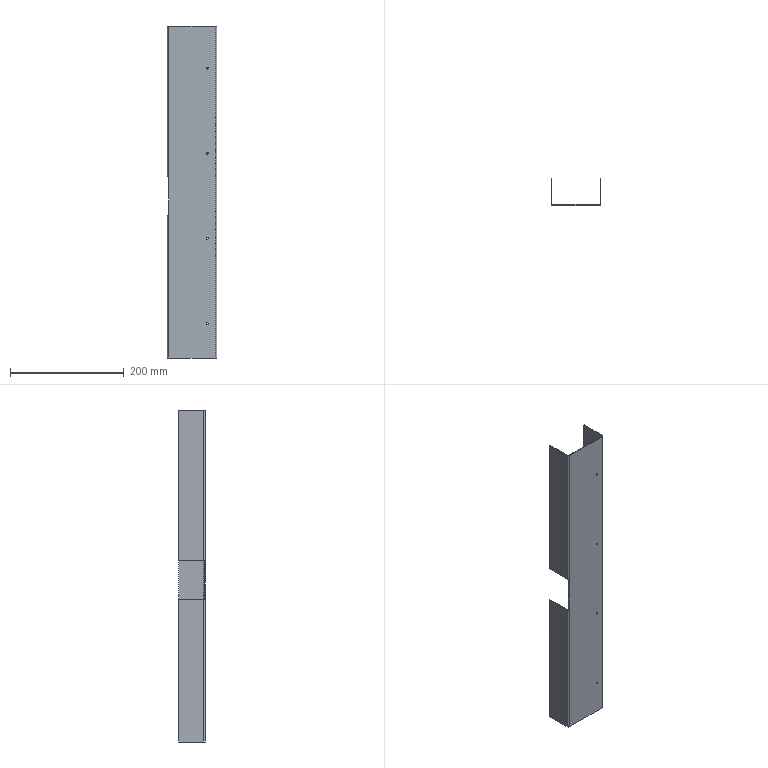Part | SolidWorks | features ICE 2, Cut 1, FlatPattern 1, SMBaseFlange 1, SheetMetal 1 | 1 solid | 38 faces | box 88 x 47.5 x 585 mm | volume 151349 mm3 | plane 24 | cylinder 14 | commonest cylinder face diameters 3 x11 6 x3
STEP:
#1=CARTESIAN_POINT('',(57.727,5.741,59.2));
#2=VERTEX_POINT('',#1);
#3=CARTESIAN_POINT('',(57.727,5.741,62.2));
#4=VERTEX_POINT('',#3);
#5=CARTESIAN_POINT('',(57.727,5.741,60.7));
#6=DIRECTION('',(0.,1.,0.));
#7=DIRECTION('',(0.,0.,1.));
#8=AXIS2_PLACEMENT_3D('',#5,#6,#7);
#9=CIRCLE('',#8,1.5);
#10=EDGE_CURVE('',#2,#4,#9,.T.);
#11=ORIENTED_EDGE('',*,*,#10,.T.);
#12=CARTESIAN_POINT('',(57.727,4.241,62.2));
#13=VERTEX_POINT('',#12);
#14=CARTESIAN_POINT('',(57.727,14.241,62.2));
#15=DIRECTION('',(0.,-1.,0.));
#16=VECTOR('',#15,1000.);
#17=LINE('',#14,#16);
#18=EDGE_CURVE('',#4,#13,#17,.T.);
#19=ORIENTED_EDGE('',*,*,#18,.T.);
#20=CARTESIAN_POINT('',(57.727,4.241,59.2));
#21=VERTEX_POINT('',#20);
#22=CARTESIAN_POINT('',(57.727,4.241,60.7));
#23=DIRECTION('',(0.,-1.,0.));
#24=DIRECTION('',(0.,0.,-1.));
#25=AXIS2_PLACEMENT_3D('',#22,#23,#24);
#26=CIRCLE('',#25,1.5);
#27=EDGE_CURVE('',#13,#21,#26,.T.);
#28=ORIENTED_EDGE('',*,*,#27,.T.);
#29=CARTESIAN_POINT('',(57.727,14.241,59.2));
#30=DIRECTION('',(0.,-1.,0.));
#31=VECTOR('',#30,1000.);
#32=LINE('',#29,#31);
#33=EDGE_CURVE('',#2,#21,#32,.T.);
#34=ORIENTED_EDGE('',*,*,#33,.F.);
#35=EDGE_LOOP('',(#11,#19,#28,#34));
#36=FACE_OUTER_BOUND('',#35,.T.);
#37=CARTESIAN_POINT('',(57.727,14.241,60.7));
#38=DIRECTION('',(0.,-1.,0.));
#39=DIRECTION('',(0.,0.,-1.));
#40=AXIS2_PLACEMENT_3D('',#37,#38,#39);
#41=CYLINDRICAL_SURFACE('',#40,1.5);
#42=ADVANCED_FACE('',(#36),#41,.F.);
#43=CARTESIAN_POINT('',(57.727,5.741,209.2));
#44=VERTEX_POINT('',#43);
#45=CARTESIAN_POINT('',(57.727,5.741,212.2));
#46=VERTEX_POINT('',#45);
#47=CARTESIAN_POINT('',(57.727,5.741,210.7));
#48=DIRECTION('',(0.,1.,0.));
#49=DIRECTION('',(0.,0.,1.));
#50=AXIS2_PLACEMENT_3D('',#47,#48,#49);
#51=CIRCLE('',#50,1.5);
#52=EDGE_CURVE('',#44,#46,#51,.T.);
#53=ORIENTED_EDGE('',*,*,#52,.T.);
#54=CARTESIAN_POINT('',(57.727,4.241,212.2));
#55=VERTEX_POINT('',#54);
#56=CARTESIAN_POINT('',(57.727,14.241,212.2));
#57=DIRECTION('',(0.,-1.,0.));
#58=VECTOR('',#57,1000.);
#59=LINE('',#56,#58);
#60=EDGE_CURVE('',#46,#55,#59,.T.);
#61=ORIENTED_EDGE('',*,*,#60,.T.);
#62=CARTESIAN_POINT('',(57.727,4.241,209.2));
#63=VERTEX_POINT('',#62);
#64=CARTESIAN_POINT('',(57.727,4.241,210.7));
#65=DIRECTION('',(0.,-1.,0.));
#66=DIRECTION('',(0.,0.,-1.));
#67=AXIS2_PLACEMENT_3D('',#64,#65,#66);
#68=CIRCLE('',#67,1.5);
#69=EDGE_CURVE('',#55,#63,#68,.T.);
#70=ORIENTED_EDGE('',*,*,#69,.T.);
#71=CARTESIAN_POINT('',(57.727,14.241,209.2));
#72=DIRECTION('',(0.,-1.,0.));
#73=VECTOR('',#72,1000.);
#74=LINE('',#71,#73);
#75=EDGE_CURVE('',#44,#63,#74,.T.);
#76=ORIENTED_EDGE('',*,*,#75,.F.);
#77=EDGE_LOOP('',(#53,#61,#70,#76));
#78=FACE_OUTER_BOUND('',#77,.T.);
#79=CARTESIAN_POINT('',(57.727,14.241,210.7));
#80=DIRECTION('',(0.,-1.,0.));
#81=DIRECTION('',(0.,0.,-1.));
#82=AXIS2_PLACEMENT_3D('',#79,#80,#81);
#83=CYLINDRICAL_SURFACE('',#82,1.5);
#84=ADVANCED_FACE('',(#78),#83,.F.);
#85=CARTESIAN_POINT('',(57.727,5.741,359.2));
#86=VERTEX_POINT('',#85);
#87=CARTESIAN_POINT('',(57.727,5.741,362.2));
#88=VERTEX_POINT('',#87);
#89=CARTESIAN_POINT('',(57.727,5.741,360.7));
#90=DIRECTION('',(0.,1.,0.));
#91=DIRECTION('',(0.,0.,1.));
#92=AXIS2_PLACEMENT_3D('',#89,#90,#91);
#93=CIRCLE('',#92,1.5);
#94=EDGE_CURVE('',#86,#88,#93,.T.);
#95=ORIENTED_EDGE('',*,*,#94,.T.);
#96=CARTESIAN_POINT('',(57.727,4.241,362.2));
#97=VERTEX_POINT('',#96);
#98=CARTESIAN_POINT('',(57.727,14.241,362.2));
#99=DIRECTION('',(0.,-1.,0.));
#100=VECTOR('',#99,1000.);
#101=LINE('',#98,#100);
#102=EDGE_CURVE('',#88,#97,#101,.T.);
#103=ORIENTED_EDGE('',*,*,#102,.T.);
#104=CARTESIAN_POINT('',(57.727,4.241,359.2));
#105=VERTEX_POINT('',#104);
#106=CARTESIAN_POINT('',(57.727,4.241,360.7));
#107=DIRECTION('',(0.,-1.,0.));
#108=DIRECTION('',(0.,0.,-1.));
#109=AXIS2_PLACEMENT_3D('',#106,#107,#108);
#110=CIRCLE('',#109,1.5);
#111=EDGE_CURVE('',#97,#105,#110,.T.);
#112=ORIENTED_EDGE('',*,*,#111,.T.);
#113=CARTESIAN_POINT('',(57.727,14.241,359.2));
#114=DIRECTION('',(0.,-1.,0.));
#115=VECTOR('',#114,1000.);
#116=LINE('',#113,#115);
#117=EDGE_CURVE('',#86,#105,#116,.T.);
#118=ORIENTED_EDGE('',*,*,#117,.F.);
#119=EDGE_LOOP('',(#95,#103,#112,#118));
#120=FACE_OUTER_BOUND('',#119,.T.);
#121=CARTESIAN_POINT('',(57.727,14.241,360.7));
#122=DIRECTION('',(0.,-1.,0.));
#123=DIRECTION('',(0.,0.,-1.));
#124=AXIS2_PLACEMENT_3D('',#121,#122,#123);
#125=CYLINDRICAL_SURFACE('',#124,1.5);
#126=ADVANCED_FACE('',(#120),#125,.F.);
#127=CARTESIAN_POINT('',(57.727,5.741,509.2));
#128=VERTEX_POINT('',#127);
#129=CARTESIAN_POINT('',(57.727,5.741,512.2));
#130=VERTEX_POINT('',#129);
#131=CARTESIAN_POINT('',(57.727,5.741,510.7));
#132=DIRECTION('',(0.,1.,0.));
#133=DIRECTION('',(0.,0.,1.));
#134=AXIS2_PLACEMENT_3D('',#131,#132,#133);
#135=CIRCLE('',#134,1.5);
#136=EDGE_CURVE('',#128,#130,#135,.T.);
#137=ORIENTED_EDGE('',*,*,#136,.T.);
#138=CARTESIAN_POINT('',(57.727,4.241,512.2));
#139=VERTEX_POINT('',#138);
#140=CARTESIAN_POINT('',(57.727,14.241,512.2));
#141=DIRECTION('',(0.,-1.,0.));
#142=VECTOR('',#141,1000.);
#143=LINE('',#140,#142);
#144=EDGE_CURVE('',#130,#139,#143,.T.);
#145=ORIENTED_EDGE('',*,*,#144,.T.);
#146=CARTESIAN_POINT('',(57.727,4.241,509.2));
#147=VERTEX_POINT('',#146);
#148=CARTESIAN_POINT('',(57.727,4.241,510.7));
#149=DIRECTION('',(0.,-1.,0.));
#150=DIRECTION('',(0.,0.,-1.));
#151=AXIS2_PLACEMENT_3D('',#148,#149,#150);
#152=CIRCLE('',#151,1.5);
#153=EDGE_CURVE('',#139,#147,#152,.T.);
#154=ORIENTED_EDGE('',*,*,#153,.T.);
#155=CARTESIAN_POINT('',(57.727,14.241,509.2));
#156=DIRECTION('',(0.,-1.,0.));
#157=VECTOR('',#156,1000.);
#158=LINE('',#155,#157);
#159=EDGE_CURVE('',#128,#147,#158,.T.);
#160=ORIENTED_EDGE('',*,*,#159,.F.);
#161=EDGE_LOOP('',(#137,#145,#154,#160));
#162=FACE_OUTER_BOUND('',#161,.T.);
#163=CARTESIAN_POINT('',(57.727,14.241,510.7));
#164=DIRECTION('',(0.,-1.,0.));
#165=DIRECTION('',(0.,0.,-1.));
#166=AXIS2_PLACEMENT_3D('',#163,#164,#165);
#167=CYLINDRICAL_SURFACE('',#166,1.5);
#168=ADVANCED_FACE('',(#162),#167,.F.);
#169=CARTESIAN_POINT('',(-13.373,7.241,319.25));
#170=VERTEX_POINT('',#169);
#171=CARTESIAN_POINT('',(-10.373,4.241,319.25));
#172=VERTEX_POINT('',#171);
#173=CARTESIAN_POINT('',(-10.373,7.241,319.25));
#174=DIRECTION('',(0.,0.,1.));
#175=DIRECTION('',(1.,0.,0.));
#176=AXIS2_PLACEMENT_3D('',#173,#174,#175);
#177=CIRCLE('',#176,3.);
#178=EDGE_CURVE('',#170,#172,#177,.T.);
#179=ORIENTED_EDGE('',*,*,#178,.T.);
#180=CARTESIAN_POINT('',(-10.373,4.241,585.));
#181=VERTEX_POINT('',#180);
#182=CARTESIAN_POINT('',(-10.373,4.241,585.));
#183=DIRECTION('',(0.,0.,-1.));
#184=VECTOR('',#183,1000.);
#185=LINE('',#182,#184);
#186=EDGE_CURVE('',#181,#172,#185,.T.);
#187=ORIENTED_EDGE('',*,*,#186,.F.);
#188=CARTESIAN_POINT('',(-13.373,7.241,585.));
#189=VERTEX_POINT('',#188);
#190=CARTESIAN_POINT('',(-10.373,7.241,585.));
#191=DIRECTION('',(0.,0.,1.));
#192=DIRECTION('',(1.,0.,0.));
#193=AXIS2_PLACEMENT_3D('',#190,#191,#192);
#194=CIRCLE('',#193,3.);
#195=EDGE_CURVE('',#189,#181,#194,.T.);
#196=ORIENTED_EDGE('',*,*,#195,.F.);
#197=CARTESIAN_POINT('',(-13.373,7.241,585.));
#198=DIRECTION('',(0.,0.,-1.));
#199=VECTOR('',#198,1000.);
#200=LINE('',#197,#199);
#201=EDGE_CURVE('',#189,#170,#200,.T.);
#202=ORIENTED_EDGE('',*,*,#201,.T.);
#203=EDGE_LOOP('',(#179,#187,#196,#202));
#204=FACE_OUTER_BOUND('',#203,.T.);
#205=CARTESIAN_POINT('',(-10.373,7.241,585.));
#206=DIRECTION('',(0.,0.,-1.));
#207=DIRECTION('',(-1.,0.,0.));
#208=AXIS2_PLACEMENT_3D('',#205,#206,#207);
#209=CYLINDRICAL_SURFACE('',#208,3.);
#210=ADVANCED_FACE('',(#204),#209,.T.);
#211=CARTESIAN_POINT('',(-10.373,5.741,251.75));
#212=VERTEX_POINT('',#211);
#213=CARTESIAN_POINT('',(-11.873,7.241,251.75));
#214=VERTEX_POINT('',#213);
#215=CARTESIAN_POINT('',(-10.373,7.241,251.75));
#216=DIRECTION('',(0.,0.,-1.));
#217=DIRECTION('',(-1.,0.,0.));
#218=AXIS2_PLACEMENT_3D('',#215,#216,#217);
#219=CIRCLE('',#218,1.5);
#220=EDGE_CURVE('',#212,#214,#219,.T.);
#221=ORIENTED_EDGE('',*,*,#220,.F.);
#222=CARTESIAN_POINT('',(-10.373,5.741,0.));
#223=VERTEX_POINT('',#222);
#224=CARTESIAN_POINT('',(-10.373,5.741,585.));
#225=DIRECTION('',(0.,0.,-1.));
#226=VECTOR('',#225,1000.);
#227=LINE('',#224,#226);
#228=EDGE_CURVE('',#212,#223,#227,.T.);
#229=ORIENTED_EDGE('',*,*,#228,.T.);
#230=CARTESIAN_POINT('',(-11.873,7.241,0.));
#231=VERTEX_POINT('',#230);
#232=CARTESIAN_POINT('',(-10.373,7.241,0.));
#233=DIRECTION('',(0.,0.,1.));
#234=DIRECTION('',(-1.,0.,0.));
#235=AXIS2_PLACEMENT_3D('',#232,#233,#234);
#236=CIRCLE('',#235,1.5);
#237=EDGE_CURVE('',#231,#223,#236,.T.);
#238=ORIENTED_EDGE('',*,*,#237,.F.);
#239=CARTESIAN_POINT('',(-11.873,7.241,585.));
#240=DIRECTION('',(0.,0.,-1.));
#241=VECTOR('',#240,1000.);
#242=LINE('',#239,#241);
#243=EDGE_CURVE('',#214,#231,#242,.T.);
#244=ORIENTED_EDGE('',*,*,#243,.F.);
#245=EDGE_LOOP('',(#221,#229,#238,#244));
#246=FACE_OUTER_BOUND('',#245,.T.);
#247=CARTESIAN_POINT('',(-10.373,7.241,585.));
#248=DIRECTION('',(0.,0.,-1.));
#249=DIRECTION('',(-1.,0.,0.));
#250=AXIS2_PLACEMENT_3D('',#247,#248,#249);
#251=CYLINDRICAL_SURFACE('',#250,1.5);
#252=ADVANCED_FACE('',(#246),#251,.F.);
#253=CARTESIAN_POINT('',(-11.873,51.741,251.75));
#254=VERTEX_POINT('',#253);
#255=CARTESIAN_POINT('',(-11.873,51.741,251.75));
#256=DIRECTION('',(0.,1.,0.));
#257=VECTOR('',#256,1000.);
#258=LINE('',#255,#257);
#259=EDGE_CURVE('',#214,#254,#258,.T.);
#260=ORIENTED_EDGE('',*,*,#259,.F.);
#261=ORIENTED_EDGE('',*,*,#243,.T.);
#262=CARTESIAN_POINT('',(-11.873,51.741,0.));
#263=VERTEX_POINT('',#262);
#264=CARTESIAN_POINT('',(-11.873,51.741,0.));
#265=DIRECTION('',(0.,-1.,0.));
#266=VECTOR('',#265,1000.);
#267=LINE('',#264,#266);
#268=EDGE_CURVE('',#263,#231,#267,.T.);
#269=ORIENTED_EDGE('',*,*,#268,.F.);
#270=CARTESIAN_POINT('',(-11.873,51.741,585.));
#271=DIRECTION('',(0.,0.,-1.));
#272=VECTOR('',#271,1000.);
#273=LINE('',#270,#272);
#274=EDGE_CURVE('',#254,#263,#273,.T.);
#275=ORIENTED_EDGE('',*,*,#274,.F.);
#276=EDGE_LOOP('',(#260,#261,#269,#275));
#277=FACE_OUTER_BOUND('',#276,.T.);
#278=CARTESIAN_POINT('',(-11.873,51.741,585.));
#279=DIRECTION('',(1.,0.,0.));
#280=DIRECTION('',(0.,1.,0.));
#281=AXIS2_PLACEMENT_3D('',#278,#279,#280);
#282=PLANE('',#281);
#283=ADVANCED_FACE('',(#277),#282,.T.);
#284=CARTESIAN_POINT('',(-13.373,51.741,251.75));
#285=VERTEX_POINT('',#284);
#286=CARTESIAN_POINT('',(-110.672,51.741,251.75));
#287=DIRECTION('',(-1.,0.,0.));
#288=VECTOR('',#287,1000.);
#289=LINE('',#286,#288);
#290=EDGE_CURVE('',#254,#285,#289,.T.);
#291=ORIENTED_EDGE('',*,*,#290,.F.);
#292=ORIENTED_EDGE('',*,*,#274,.T.);
#293=CARTESIAN_POINT('',(-13.373,51.741,0.));
#294=VERTEX_POINT('',#293);
#295=CARTESIAN_POINT('',(-13.373,51.741,0.));
#296=DIRECTION('',(1.,0.,0.));
#297=VECTOR('',#296,1000.);
#298=LINE('',#295,#297);
#299=EDGE_CURVE('',#294,#263,#298,.T.);
#300=ORIENTED_EDGE('',*,*,#299,.F.);
#301=CARTESIAN_POINT('',(-13.373,51.741,585.));
#302=DIRECTION('',(0.,0.,-1.));
#303=VECTOR('',#302,1000.);
#304=LINE('',#301,#303);
#305=EDGE_CURVE('',#285,#294,#304,.T.);
#306=ORIENTED_EDGE('',*,*,#305,.F.);
#307=EDGE_LOOP('',(#291,#292,#300,#306));
#308=FACE_OUTER_BOUND('',#307,.T.);
#309=CARTESIAN_POINT('',(-13.373,51.741,585.));
#310=DIRECTION('',(0.,1.,0.));
#311=DIRECTION('',(0.,0.,1.));
#312=AXIS2_PLACEMENT_3D('',#309,#310,#311);
#313=PLANE('',#312);
#314=ADVANCED_FACE('',(#308),#313,.T.);
#315=CARTESIAN_POINT('',(-13.373,7.241,251.75));
#316=VERTEX_POINT('',#315);
#317=CARTESIAN_POINT('',(-13.373,7.241,0.));
#318=VERTEX_POINT('',#317);
#319=CARTESIAN_POINT('',(-13.373,7.241,585.));
#320=DIRECTION('',(0.,0.,-1.));
#321=VECTOR('',#320,1000.);
#322=LINE('',#319,#321);
#323=EDGE_CURVE('',#316,#318,#322,.T.);
#324=ORIENTED_EDGE('',*,*,#323,.F.);
#325=CARTESIAN_POINT('',(-13.373,51.741,251.75));
#326=DIRECTION('',(0.,1.,0.));
#327=VECTOR('',#326,1000.);
#328=LINE('',#325,#327);
#329=EDGE_CURVE('',#316,#285,#328,.T.);
#330=ORIENTED_EDGE('',*,*,#329,.T.);
#331=ORIENTED_EDGE('',*,*,#305,.T.);
#332=CARTESIAN_POINT('',(-13.373,51.741,0.));
#333=DIRECTION('',(0.,-1.,0.));
#334=VECTOR('',#333,1000.);
#335=LINE('',#332,#334);
#336=EDGE_CURVE('',#294,#318,#335,.T.);
#337=ORIENTED_EDGE('',*,*,#336,.T.);
#338=EDGE_LOOP('',(#324,#330,#331,#337));
#339=FACE_OUTER_BOUND('',#338,.T.);
#340=CARTESIAN_POINT('',(-13.373,51.741,585.));
#341=DIRECTION('',(1.,0.,0.));
#342=DIRECTION('',(0.,1.,0.));
#343=AXIS2_PLACEMENT_3D('',#340,#341,#342);
#344=PLANE('',#343);
#345=ADVANCED_FACE('',(#339),#344,.F.);
#346=CARTESIAN_POINT('',(-10.373,5.741,585.));
#347=VERTEX_POINT('',#346);
#348=CARTESIAN_POINT('',(-10.373,5.741,585.));
#349=DIRECTION('',(0.,-1.,0.));
#350=VECTOR('',#349,1000.);
#351=LINE('',#348,#350);
#352=EDGE_CURVE('',#347,#181,#351,.T.);
#353=ORIENTED_EDGE('',*,*,#352,.F.);
#354=CARTESIAN_POINT('',(-11.873,7.241,585.));
#355=VERTEX_POINT('',#354);
#356=CARTESIAN_POINT('',(-10.373,7.241,585.));
#357=DIRECTION('',(0.,0.,1.));
#358=DIRECTION('',(-1.,0.,0.));
#359=AXIS2_PLACEMENT_3D('',#356,#357,#358);
#360=CIRCLE('',#359,1.5);
#361=EDGE_CURVE('',#355,#347,#360,.T.);
#362=ORIENTED_EDGE('',*,*,#361,.F.);
#363=CARTESIAN_POINT('',(-13.373,7.241,585.));
#364=DIRECTION('',(1.,0.,0.));
#365=VECTOR('',#364,1000.);
#366=LINE('',#363,#365);
#367=EDGE_CURVE('',#189,#355,#366,.T.);
#368=ORIENTED_EDGE('',*,*,#367,.F.);
#369=ORIENTED_EDGE('',*,*,#195,.T.);
#370=EDGE_LOOP('',(#353,#362,#368,#369));
#371=FACE_OUTER_BOUND('',#370,.T.);
#372=CARTESIAN_POINT('',(-10.373,5.741,585.));
#373=DIRECTION('',(0.,0.,1.));
#374=DIRECTION('',(1.,0.,0.));
#375=AXIS2_PLACEMENT_3D('',#372,#373,#374);
#376=PLANE('',#375);
#377=ADVANCED_FACE('',(#371),#376,.T.);
#378=CARTESIAN_POINT('',(71.627,5.741,585.));
#379=VERTEX_POINT('',#378);
#380=CARTESIAN_POINT('',(-11.873,5.741,585.));
#381=DIRECTION('',(1.,0.,0.));
#382=VECTOR('',#381,1000.);
#383=LINE('',#380,#382);
#384=EDGE_CURVE('',#347,#379,#383,.T.);
#385=ORIENTED_EDGE('',*,*,#384,.F.);
#386=ORIENTED_EDGE('',*,*,#352,.T.);
#387=CARTESIAN_POINT('',(71.627,4.241,585.));
#388=VERTEX_POINT('',#387);
#389=CARTESIAN_POINT('',(-11.873,4.241,585.));
#390=DIRECTION('',(1.,0.,0.));
#391=VECTOR('',#390,1000.);
#392=LINE('',#389,#391);
#393=EDGE_CURVE('',#181,#388,#392,.T.);
#394=ORIENTED_EDGE('',*,*,#393,.T.);
#395=CARTESIAN_POINT('',(71.627,4.241,585.));
#396=DIRECTION('',(0.,1.,0.));
#397=VECTOR('',#396,1000.);
#398=LINE('',#395,#397);
#399=EDGE_CURVE('',#388,#379,#398,.T.);
#400=ORIENTED_EDGE('',*,*,#399,.T.);
#401=EDGE_LOOP('',(#385,#386,#394,#400));
#402=FACE_OUTER_BOUND('',#401,.T.);
#403=CARTESIAN_POINT('',(-13.373,7.241,585.));
#404=DIRECTION('',(0.,0.,1.));
#405=DIRECTION('',(1.,0.,0.));
#406=AXIS2_PLACEMENT_3D('',#403,#404,#405);
#407=PLANE('',#406);
#408=ADVANCED_FACE('',(#402),#407,.T.);
#409=CARTESIAN_POINT('',(-11.873,7.241,0.));
#410=DIRECTION('',(-1.,0.,0.));
#411=VECTOR('',#410,1000.);
#412=LINE('',#409,#411);
#413=EDGE_CURVE('',#231,#318,#412,.T.);
#414=ORIENTED_EDGE('',*,*,#413,.F.);
#415=ORIENTED_EDGE('',*,*,#237,.T.);
#416=CARTESIAN_POINT('',(-10.373,4.241,0.));
#417=VERTEX_POINT('',#416);
#418=CARTESIAN_POINT('',(-10.373,4.241,0.));
#419=DIRECTION('',(0.,1.,0.));
#420=VECTOR('',#419,1000.);
#421=LINE('',#418,#420);
#422=EDGE_CURVE('',#417,#223,#421,.T.);
#423=ORIENTED_EDGE('',*,*,#422,.F.);
#424=CARTESIAN_POINT('',(-10.373,7.241,0.));
#425=DIRECTION('',(0.,0.,1.));
#426=DIRECTION('',(1.,0.,0.));
#427=AXIS2_PLACEMENT_3D('',#424,#425,#426);
#428=CIRCLE('',#427,3.);
#429=EDGE_CURVE('',#318,#417,#428,.T.);
#430=ORIENTED_EDGE('',*,*,#429,.F.);
#431=EDGE_LOOP('',(#414,#415,#423,#430));
#432=FACE_OUTER_BOUND('',#431,.T.);
#433=CARTESIAN_POINT('',(-11.873,7.241,0.));
#434=DIRECTION('',(0.,0.,-1.));
#435=DIRECTION('',(-1.,0.,0.));
#436=AXIS2_PLACEMENT_3D('',#433,#434,#435);
#437=PLANE('',#436);
#438=ADVANCED_FACE('',(#432),#437,.T.);
#439=ORIENTED_EDGE('',*,*,#268,.T.);
#440=ORIENTED_EDGE('',*,*,#413,.T.);
#441=ORIENTED_EDGE('',*,*,#336,.F.);
#442=ORIENTED_EDGE('',*,*,#299,.T.);
#443=EDGE_LOOP('',(#439,#440,#441,#442));
#444=FACE_OUTER_BOUND('',#443,.T.);
#445=CARTESIAN_POINT('',(-10.373,4.241,0.));
#446=DIRECTION('',(0.,0.,-1.));
#447=DIRECTION('',(-1.,0.,0.));
#448=AXIS2_PLACEMENT_3D('',#445,#446,#447);
#449=PLANE('',#448);
#450=ADVANCED_FACE('',(#444),#449,.T.);
#451=CARTESIAN_POINT('',(73.127,7.241,585.));
#452=VERTEX_POINT('',#451);
#453=CARTESIAN_POINT('',(74.627,7.241,585.));
#454=VERTEX_POINT('',#453);
#455=CARTESIAN_POINT('',(73.127,7.241,585.));
#456=DIRECTION('',(1.,0.,0.));
#457=VECTOR('',#456,1000.);
#458=LINE('',#455,#457);
#459=EDGE_CURVE('',#452,#454,#458,.T.);
#460=ORIENTED_EDGE('',*,*,#459,.F.);
#461=CARTESIAN_POINT('',(71.627,7.241,585.));
#462=DIRECTION('',(0.,0.,1.));
#463=DIRECTION('',(-1.,0.,0.));
#464=AXIS2_PLACEMENT_3D('',#461,#462,#463);
#465=CIRCLE('',#464,1.5);
#466=EDGE_CURVE('',#379,#452,#465,.T.);
#467=ORIENTED_EDGE('',*,*,#466,.F.);
#468=ORIENTED_EDGE('',*,*,#399,.F.);
#469=CARTESIAN_POINT('',(71.627,7.241,585.));
#470=DIRECTION('',(0.,0.,1.));
#471=DIRECTION('',(1.,0.,0.));
#472=AXIS2_PLACEMENT_3D('',#469,#470,#471);
#473=CIRCLE('',#472,3.);
#474=EDGE_CURVE('',#388,#454,#473,.T.);
#475=ORIENTED_EDGE('',*,*,#474,.T.);
#476=EDGE_LOOP('',(#460,#467,#468,#475));
#477=FACE_OUTER_BOUND('',#476,.T.);
#478=CARTESIAN_POINT('',(73.127,7.241,585.));
#479=DIRECTION('',(0.,0.,1.));
#480=DIRECTION('',(1.,0.,0.));
#481=AXIS2_PLACEMENT_3D('',#478,#479,#480);
#482=PLANE('',#481);
#483=ADVANCED_FACE('',(#477),#482,.T.);
#484=CARTESIAN_POINT('',(73.127,51.741,585.));
#485=VERTEX_POINT('',#484);
#486=CARTESIAN_POINT('',(73.127,5.741,585.));
#487=DIRECTION('',(0.,1.,0.));
#488=VECTOR('',#487,1000.);
#489=LINE('',#486,#488);
#490=EDGE_CURVE('',#452,#485,#489,.T.);
#491=ORIENTED_EDGE('',*,*,#490,.F.);
#492=ORIENTED_EDGE('',*,*,#459,.T.);
#493=CARTESIAN_POINT('',(74.627,51.741,585.));
#494=VERTEX_POINT('',#493);
#495=CARTESIAN_POINT('',(74.627,5.741,585.));
#496=DIRECTION('',(0.,1.,0.));
#497=VECTOR('',#496,1000.);
#498=LINE('',#495,#497);
#499=EDGE_CURVE('',#454,#494,#498,.T.);
#500=ORIENTED_EDGE('',*,*,#499,.T.);
#501=CARTESIAN_POINT('',(73.127,51.741,585.));
#502=DIRECTION('',(1.,0.,0.));
#503=VECTOR('',#502,1000.);
#504=LINE('',#501,#503);
#505=EDGE_CURVE('',#485,#494,#504,.T.);
#506=ORIENTED_EDGE('',*,*,#505,.F.);
#507=EDGE_LOOP('',(#491,#492,#500,#506));
#508=FACE_OUTER_BOUND('',#507,.T.);
#509=CARTESIAN_POINT('',(71.627,4.241,585.));
#510=DIRECTION('',(0.,0.,1.));
#511=DIRECTION('',(1.,0.,0.));
#512=AXIS2_PLACEMENT_3D('',#509,#510,#511);
#513=PLANE('',#512);
#514=ADVANCED_FACE('',(#508),#513,.T.);
#515=CARTESIAN_POINT('',(71.627,5.741,0.));
#516=VERTEX_POINT('',#515);
#517=CARTESIAN_POINT('',(71.627,4.241,0.));
#518=VERTEX_POINT('',#517);
#519=CARTESIAN_POINT('',(71.627,5.741,0.));
#520=DIRECTION('',(0.,-1.,0.));
#521=VECTOR('',#520,1000.);
#522=LINE('',#519,#521);
#523=EDGE_CURVE('',#516,#518,#522,.T.);
#524=ORIENTED_EDGE('',*,*,#523,.F.);
#525=CARTESIAN_POINT('',(73.127,7.241,0.));
#526=VERTEX_POINT('',#525);
#527=CARTESIAN_POINT('',(71.627,7.241,0.));
#528=DIRECTION('',(0.,0.,1.));
#529=DIRECTION('',(-1.,0.,0.));
#530=AXIS2_PLACEMENT_3D('',#527,#528,#529);
#531=CIRCLE('',#530,1.5);
#532=EDGE_CURVE('',#516,#526,#531,.T.);
#533=ORIENTED_EDGE('',*,*,#532,.T.);
#534=CARTESIAN_POINT('',(74.627,7.241,0.));
#535=VERTEX_POINT('',#534);
#536=CARTESIAN_POINT('',(74.627,7.241,0.));
#537=DIRECTION('',(-1.,0.,0.));
#538=VECTOR('',#537,1000.);
#539=LINE('',#536,#538);
#540=EDGE_CURVE('',#535,#526,#539,.T.);
#541=ORIENTED_EDGE('',*,*,#540,.F.);
#542=CARTESIAN_POINT('',(71.627,7.241,0.));
#543=DIRECTION('',(0.,0.,1.));
#544=DIRECTION('',(1.,0.,0.));
#545=AXIS2_PLACEMENT_3D('',#542,#543,#544);
#546=CIRCLE('',#545,3.);
#547=EDGE_CURVE('',#518,#535,#546,.T.);
#548=ORIENTED_EDGE('',*,*,#547,.F.);
#549=EDGE_LOOP('',(#524,#533,#541,#548));
#550=FACE_OUTER_BOUND('',#549,.T.);
#551=CARTESIAN_POINT('',(71.627,5.741,0.));
#552=DIRECTION('',(0.,0.,-1.));
#553=DIRECTION('',(-1.,0.,0.));
#554=AXIS2_PLACEMENT_3D('',#551,#552,#553);
#555=PLANE('',#554);
#556=ADVANCED_FACE('',(#550),#555,.T.);
#557=CARTESIAN_POINT('',(-11.873,5.741,0.));
#558=DIRECTION('',(1.,0.,0.));
#559=VECTOR('',#558,1000.);
#560=LINE('',#557,#559);
#561=EDGE_CURVE('',#223,#516,#560,.T.);
#562=ORIENTED_EDGE('',*,*,#561,.T.);
#563=ORIENTED_EDGE('',*,*,#523,.T.);
#564=CARTESIAN_POINT('',(-11.873,4.241,0.));
#565=DIRECTION('',(1.,0.,0.));
#566=VECTOR('',#565,1000.);
#567=LINE('',#564,#566);
#568=EDGE_CURVE('',#417,#518,#567,.T.);
#569=ORIENTED_EDGE('',*,*,#568,.F.);
#570=ORIENTED_EDGE('',*,*,#422,.T.);
#571=EDGE_LOOP('',(#562,#563,#569,#570));
#572=FACE_OUTER_BOUND('',#571,.T.);
#573=CARTESIAN_POINT('',(74.627,7.241,0.));
#574=DIRECTION('',(0.,0.,-1.));
#575=DIRECTION('',(-1.,0.,0.));
#576=AXIS2_PLACEMENT_3D('',#573,#574,#575);
#577=PLANE('',#576);
#578=ADVANCED_FACE('',(#572),#577,.T.);
#579=CARTESIAN_POINT('',(74.627,51.741,0.));
#580=VERTEX_POINT('',#579);
#581=CARTESIAN_POINT('',(74.627,5.741,0.));
#582=DIRECTION('',(0.,1.,0.));
#583=VECTOR('',#582,1000.);
#584=LINE('',#581,#583);
#585=EDGE_CURVE('',#535,#580,#584,.T.);
#586=ORIENTED_EDGE('',*,*,#585,.T.);
#587=CARTESIAN_POINT('',(74.627,51.741,585.));
#588=DIRECTION('',(0.,0.,-1.));
#589=VECTOR('',#588,1000.);
#590=LINE('',#587,#589);
#591=EDGE_CURVE('',#494,#580,#590,.T.);
#592=ORIENTED_EDGE('',*,*,#591,.F.);
#593=ORIENTED_EDGE('',*,*,#499,.F.);
#594=CARTESIAN_POINT('',(74.627,7.241,585.));
#595=DIRECTION('',(0.,0.,-1.));
#596=VECTOR('',#595,1000.);
#597=LINE('',#594,#596);
#598=EDGE_CURVE('',#454,#535,#597,.T.);
#599=ORIENTED_EDGE('',*,*,#598,.T.);
#600=EDGE_LOOP('',(#586,#592,#593,#599));
#601=FACE_OUTER_BOUND('',#600,.T.);
#602=CARTESIAN_POINT('',(74.627,5.741,585.));
#603=DIRECTION('',(-1.,0.,0.));
#604=DIRECTION('',(0.,0.,1.));
#605=AXIS2_PLACEMENT_3D('',#602,#603,#604);
#606=PLANE('',#605);
#607=ADVANCED_FACE('',(#601),#606,.F.);
#608=CARTESIAN_POINT('',(73.127,51.741,0.));
#609=VERTEX_POINT('',#608);
#610=CARTESIAN_POINT('',(73.127,51.741,0.));
#611=DIRECTION('',(1.,0.,0.));
#612=VECTOR('',#611,1000.);
#613=LINE('',#610,#612);
#614=EDGE_CURVE('',#609,#580,#613,.T.);
#615=ORIENTED_EDGE('',*,*,#614,.F.);
#616=CARTESIAN_POINT('',(73.127,51.741,585.));
#617=DIRECTION('',(0.,0.,-1.));
#618=VECTOR('',#617,1000.);
#619=LINE('',#616,#618);
#620=EDGE_CURVE('',#485,#609,#619,.T.);
#621=ORIENTED_EDGE('',*,*,#620,.F.);
#622=ORIENTED_EDGE('',*,*,#505,.T.);
#623=ORIENTED_EDGE('',*,*,#591,.T.);
#624=EDGE_LOOP('',(#615,#621,#622,#623));
#625=FACE_OUTER_BOUND('',#624,.T.);
#626=CARTESIAN_POINT('',(73.127,51.741,585.));
#627=DIRECTION('',(0.,1.,0.));
#628=DIRECTION('',(0.,0.,1.));
#629=AXIS2_PLACEMENT_3D('',#626,#627,#628);
#630=PLANE('',#629);
#631=ADVANCED_FACE('',(#625),#630,.T.);
#632=CARTESIAN_POINT('',(73.127,5.741,0.));
#633=DIRECTION('',(0.,1.,0.));
#634=VECTOR('',#633,1000.);
#635=LINE('',#632,#634);
#636=EDGE_CURVE('',#526,#609,#635,.T.);
#637=ORIENTED_EDGE('',*,*,#636,.F.);
#638=CARTESIAN_POINT('',(73.127,7.241,585.));
#639=DIRECTION('',(0.,0.,-1.));
#640=VECTOR('',#639,1000.);
#641=LINE('',#638,#640);
#642=EDGE_CURVE('',#452,#526,#641,.T.);
#643=ORIENTED_EDGE('',*,*,#642,.F.);
#644=ORIENTED_EDGE('',*,*,#490,.T.);
#645=ORIENTED_EDGE('',*,*,#620,.T.);
#646=EDGE_LOOP('',(#637,#643,#644,#645));
#647=FACE_OUTER_BOUND('',#646,.T.);
#648=CARTESIAN_POINT('',(73.127,5.741,585.));
#649=DIRECTION('',(-1.,0.,0.));
#650=DIRECTION('',(0.,0.,1.));
#651=AXIS2_PLACEMENT_3D('',#648,#649,#650);
#652=PLANE('',#651);
#653=ADVANCED_FACE('',(#647),#652,.T.);
#654=ORIENTED_EDGE('',*,*,#532,.F.);
#655=CARTESIAN_POINT('',(71.627,5.741,585.));
#656=DIRECTION('',(0.,0.,-1.));
#657=VECTOR('',#656,1000.);
#658=LINE('',#655,#657);
#659=EDGE_CURVE('',#379,#516,#658,.T.);
#660=ORIENTED_EDGE('',*,*,#659,.F.);
#661=ORIENTED_EDGE('',*,*,#466,.T.);
#662=ORIENTED_EDGE('',*,*,#642,.T.);
#663=EDGE_LOOP('',(#654,#660,#661,#662));
#664=FACE_OUTER_BOUND('',#663,.T.);
#665=CARTESIAN_POINT('',(71.627,7.241,585.));
#666=DIRECTION('',(0.,0.,-1.));
#667=DIRECTION('',(-1.,0.,0.));
#668=AXIS2_PLACEMENT_3D('',#665,#666,#667);
#669=CYLINDRICAL_SURFACE('',#668,1.5);
#670=ADVANCED_FACE('',(#664),#669,.F.);
#671=CARTESIAN_POINT('',(-10.373,5.741,319.25));
#672=VERTEX_POINT('',#671);
#673=CARTESIAN_POINT('',(-10.373,5.741,251.75));
#674=DIRECTION('',(0.,0.,-1.));
#675=VECTOR('',#674,1000.);
#676=LINE('',#673,#675);
#677=EDGE_CURVE('',#672,#212,#676,.T.);
#678=ORIENTED_EDGE('',*,*,#677,.F.);
#679=CARTESIAN_POINT('',(-10.373,5.741,585.));
#680=DIRECTION('',(0.,0.,-1.));
#681=VECTOR('',#680,1000.);
#682=LINE('',#679,#681);
#683=EDGE_CURVE('',#347,#672,#682,.T.);
#684=ORIENTED_EDGE('',*,*,#683,.F.);
#685=ORIENTED_EDGE('',*,*,#384,.T.);
#686=ORIENTED_EDGE('',*,*,#659,.T.);
#687=ORIENTED_EDGE('',*,*,#561,.F.);
#688=ORIENTED_EDGE('',*,*,#228,.F.);
#689=EDGE_LOOP('',(#678,#684,#685,#686,#687,#688));
#690=FACE_OUTER_BOUND('',#689,.T.);
#691=ORIENTED_EDGE('',*,*,#10,.F.);
#692=CARTESIAN_POINT('',(57.727,5.741,60.7));
#693=DIRECTION('',(0.,1.,0.));
#694=DIRECTION('',(0.,0.,1.));
#695=AXIS2_PLACEMENT_3D('',#692,#693,#694);
#696=CIRCLE('',#695,1.5);
#697=EDGE_CURVE('',#4,#2,#696,.T.);
#698=ORIENTED_EDGE('',*,*,#697,.F.);
#699=EDGE_LOOP('',(#691,#698));
#700=FACE_BOUND('',#699,.T.);
#701=ORIENTED_EDGE('',*,*,#52,.F.);
#702=CARTESIAN_POINT('',(57.727,5.741,210.7));
#703=DIRECTION('',(0.,1.,0.));
#704=DIRECTION('',(0.,0.,1.));
#705=AXIS2_PLACEMENT_3D('',#702,#703,#704);
#706=CIRCLE('',#705,1.5);
#707=EDGE_CURVE('',#46,#44,#706,.T.);
#708=ORIENTED_EDGE('',*,*,#707,.F.);
#709=EDGE_LOOP('',(#701,#708));
#710=FACE_BOUND('',#709,.T.);
#711=ORIENTED_EDGE('',*,*,#94,.F.);
#712=CARTESIAN_POINT('',(57.727,5.741,360.7));
#713=DIRECTION('',(0.,1.,0.));
#714=DIRECTION('',(0.,0.,1.));
#715=AXIS2_PLACEMENT_3D('',#712,#713,#714);
#716=CIRCLE('',#715,1.5);
#717=EDGE_CURVE('',#88,#86,#716,.T.);
#718=ORIENTED_EDGE('',*,*,#717,.F.);
#719=EDGE_LOOP('',(#711,#718));
#720=FACE_BOUND('',#719,.T.);
#721=ORIENTED_EDGE('',*,*,#136,.F.);
#722=CARTESIAN_POINT('',(57.727,5.741,510.7));
#723=DIRECTION('',(0.,1.,0.));
#724=DIRECTION('',(0.,0.,1.));
#725=AXIS2_PLACEMENT_3D('',#722,#723,#724);
#726=CIRCLE('',#725,1.5);
#727=EDGE_CURVE('',#130,#128,#726,.T.);
#728=ORIENTED_EDGE('',*,*,#727,.F.);
#729=EDGE_LOOP('',(#721,#728));
#730=FACE_BOUND('',#729,.T.);
#731=CARTESIAN_POINT('',(-11.873,5.741,585.));
#732=DIRECTION('',(0.,1.,0.));
#733=DIRECTION('',(0.,0.,1.));
#734=AXIS2_PLACEMENT_3D('',#731,#732,#733);
#735=PLANE('',#734);
#736=ADVANCED_FACE('',(#690,#700,#710,#720,#730),#735,.T.);
#737=CARTESIAN_POINT('',(-11.873,7.241,319.25));
#738=VERTEX_POINT('',#737);
#739=CARTESIAN_POINT('',(-10.373,7.241,319.25));
#740=DIRECTION('',(0.,0.,1.));
#741=DIRECTION('',(1.,0.,0.));
#742=AXIS2_PLACEMENT_3D('',#739,#740,#741);
#743=CIRCLE('',#742,1.5);
#744=EDGE_CURVE('',#738,#672,#743,.T.);
#745=ORIENTED_EDGE('',*,*,#744,.F.);
#746=CARTESIAN_POINT('',(-11.873,7.241,585.));
#747=DIRECTION('',(0.,0.,-1.));
#748=VECTOR('',#747,1000.);
#749=LINE('',#746,#748);
#750=EDGE_CURVE('',#355,#738,#749,.T.);
#751=ORIENTED_EDGE('',*,*,#750,.F.);
#752=ORIENTED_EDGE('',*,*,#361,.T.);
#753=ORIENTED_EDGE('',*,*,#683,.T.);
#754=EDGE_LOOP('',(#745,#751,#752,#753));
#755=FACE_OUTER_BOUND('',#754,.T.);
#756=CARTESIAN_POINT('',(-10.373,7.241,585.));
#757=DIRECTION('',(0.,0.,-1.));
#758=DIRECTION('',(-1.,0.,0.));
#759=AXIS2_PLACEMENT_3D('',#756,#757,#758);
#760=CYLINDRICAL_SURFACE('',#759,1.5);
#761=ADVANCED_FACE('',(#755),#760,.F.);
#762=CARTESIAN_POINT('',(-11.873,51.741,319.25));
#763=VERTEX_POINT('',#762);
#764=CARTESIAN_POINT('',(-11.873,51.741,319.25));
#765=DIRECTION('',(0.,-1.,0.));
#766=VECTOR('',#765,1000.);
#767=LINE('',#764,#766);
#768=EDGE_CURVE('',#763,#738,#767,.T.);
#769=ORIENTED_EDGE('',*,*,#768,.F.);
#770=CARTESIAN_POINT('',(-11.873,51.741,585.));
#771=VERTEX_POINT('',#770);
#772=CARTESIAN_POINT('',(-11.873,51.741,585.));
#773=DIRECTION('',(0.,0.,-1.));
#774=VECTOR('',#773,1000.);
#775=LINE('',#772,#774);
#776=EDGE_CURVE('',#771,#763,#775,.T.);
#777=ORIENTED_EDGE('',*,*,#776,.F.);
#778=CARTESIAN_POINT('',(-11.873,51.741,585.));
#779=DIRECTION('',(0.,-1.,0.));
#780=VECTOR('',#779,1000.);
#781=LINE('',#778,#780);
#782=EDGE_CURVE('',#771,#355,#781,.T.);
#783=ORIENTED_EDGE('',*,*,#782,.T.);
#784=ORIENTED_EDGE('',*,*,#750,.T.);
#785=EDGE_LOOP('',(#769,#777,#783,#784));
#786=FACE_OUTER_BOUND('',#785,.T.);
#787=CARTESIAN_POINT('',(-11.873,51.741,585.));
#788=DIRECTION('',(1.,0.,0.));
#789=DIRECTION('',(0.,1.,0.));
#790=AXIS2_PLACEMENT_3D('',#787,#788,#789);
#791=PLANE('',#790);
#792=ADVANCED_FACE('',(#786),#791,.T.);
#793=CARTESIAN_POINT('',(-13.373,51.741,319.25));
#794=VERTEX_POINT('',#793);
#795=CARTESIAN_POINT('',(-110.672,51.741,319.25));
#796=DIRECTION('',(1.,0.,0.));
#797=VECTOR('',#796,1000.);
#798=LINE('',#795,#797);
#799=EDGE_CURVE('',#794,#763,#798,.T.);
#800=ORIENTED_EDGE('',*,*,#799,.F.);
#801=CARTESIAN_POINT('',(-13.373,51.741,585.));
#802=VERTEX_POINT('',#801);
#803=CARTESIAN_POINT('',(-13.373,51.741,585.));
#804=DIRECTION('',(0.,0.,-1.));
#805=VECTOR('',#804,1000.);
#806=LINE('',#803,#805);
#807=EDGE_CURVE('',#802,#794,#806,.T.);
#808=ORIENTED_EDGE('',*,*,#807,.F.);
#809=CARTESIAN_POINT('',(-13.373,51.741,585.));
#810=DIRECTION('',(1.,0.,0.));
#811=VECTOR('',#810,1000.);
#812=LINE('',#809,#811);
#813=EDGE_CURVE('',#802,#771,#812,.T.);
#814=ORIENTED_EDGE('',*,*,#813,.T.);
#815=ORIENTED_EDGE('',*,*,#776,.T.);
#816=EDGE_LOOP('',(#800,#808,#814,#815));
#817=FACE_OUTER_BOUND('',#816,.T.);
#818=CARTESIAN_POINT('',(-13.373,51.741,585.));
#819=DIRECTION('',(0.,1.,0.));
#820=DIRECTION('',(0.,0.,1.));
#821=AXIS2_PLACEMENT_3D('',#818,#819,#820);
#822=PLANE('',#821);
#823=ADVANCED_FACE('',(#817),#822,.T.);
#824=ORIENTED_EDGE('',*,*,#807,.T.);
#825=CARTESIAN_POINT('',(-13.373,51.741,319.25));
#826=DIRECTION('',(0.,-1.,0.));
#827=VECTOR('',#826,1000.);
#828=LINE('',#825,#827);
#829=EDGE_CURVE('',#794,#170,#828,.T.);
#830=ORIENTED_EDGE('',*,*,#829,.T.);
#831=ORIENTED_EDGE('',*,*,#201,.F.);
#832=CARTESIAN_POINT('',(-13.373,51.741,585.));
#833=DIRECTION('',(0.,-1.,0.));
#834=VECTOR('',#833,1000.);
#835=LINE('',#832,#834);
#836=EDGE_CURVE('',#802,#189,#835,.T.);
#837=ORIENTED_EDGE('',*,*,#836,.F.);
#838=EDGE_LOOP('',(#824,#830,#831,#837));
#839=FACE_OUTER_BOUND('',#838,.T.);
#840=CARTESIAN_POINT('',(-13.373,51.741,585.));
#841=DIRECTION('',(1.,0.,0.));
#842=DIRECTION('',(0.,1.,0.));
#843=AXIS2_PLACEMENT_3D('',#840,#841,#842);
#844=PLANE('',#843);
#845=ADVANCED_FACE('',(#839),#844,.F.);
#846=CARTESIAN_POINT('',(-10.373,4.241,251.75));
#847=VERTEX_POINT('',#846);
#848=CARTESIAN_POINT('',(-10.373,4.241,585.));
#849=DIRECTION('',(0.,0.,-1.));
#850=VECTOR('',#849,1000.);
#851=LINE('',#848,#850);
#852=EDGE_CURVE('',#847,#417,#851,.T.);
#853=ORIENTED_EDGE('',*,*,#852,.F.);
#854=CARTESIAN_POINT('',(-10.373,7.241,251.75));
#855=DIRECTION('',(0.,0.,-1.));
#856=DIRECTION('',(-1.,0.,0.));
#857=AXIS2_PLACEMENT_3D('',#854,#855,#856);
#858=CIRCLE('',#857,3.);
#859=EDGE_CURVE('',#847,#316,#858,.T.);
#860=ORIENTED_EDGE('',*,*,#859,.T.);
#861=ORIENTED_EDGE('',*,*,#323,.T.);
#862=ORIENTED_EDGE('',*,*,#429,.T.);
#863=EDGE_LOOP('',(#853,#860,#861,#862));
#864=FACE_OUTER_BOUND('',#863,.T.);
#865=CARTESIAN_POINT('',(-10.373,7.241,585.));
#866=DIRECTION('',(0.,0.,-1.));
#867=DIRECTION('',(-1.,0.,0.));
#868=AXIS2_PLACEMENT_3D('',#865,#866,#867);
#869=CYLINDRICAL_SURFACE('',#868,3.);
#870=ADVANCED_FACE('',(#864),#869,.T.);
#871=CARTESIAN_POINT('',(57.727,4.241,60.7));
#872=DIRECTION('',(0.,-1.,0.));
#873=DIRECTION('',(0.,0.,-1.));
#874=AXIS2_PLACEMENT_3D('',#871,#872,#873);
#875=CIRCLE('',#874,1.5);
#876=EDGE_CURVE('',#21,#13,#875,.T.);
#877=ORIENTED_EDGE('',*,*,#876,.F.);
#878=ORIENTED_EDGE('',*,*,#27,.F.);
#879=EDGE_LOOP('',(#877,#878));
#880=FACE_BOUND('',#879,.T.);
#881=CARTESIAN_POINT('',(57.727,4.241,210.7));
#882=DIRECTION('',(0.,-1.,0.));
#883=DIRECTION('',(0.,0.,-1.));
#884=AXIS2_PLACEMENT_3D('',#881,#882,#883);
#885=CIRCLE('',#884,1.5);
#886=EDGE_CURVE('',#63,#55,#885,.T.);
#887=ORIENTED_EDGE('',*,*,#886,.F.);
#888=ORIENTED_EDGE('',*,*,#69,.F.);
#889=EDGE_LOOP('',(#887,#888));
#890=FACE_BOUND('',#889,.T.);
#891=CARTESIAN_POINT('',(57.727,4.241,360.7));
#892=DIRECTION('',(0.,-1.,0.));
#893=DIRECTION('',(0.,0.,-1.));
#894=AXIS2_PLACEMENT_3D('',#891,#892,#893);
#895=CIRCLE('',#894,1.5);
#896=EDGE_CURVE('',#105,#97,#895,.T.);
#897=ORIENTED_EDGE('',*,*,#896,.F.);
#898=ORIENTED_EDGE('',*,*,#111,.F.);
#899=EDGE_LOOP('',(#897,#898));
#900=FACE_BOUND('',#899,.T.);
#901=CARTESIAN_POINT('',(57.727,4.241,510.7));
#902=DIRECTION('',(0.,-1.,0.));
#903=DIRECTION('',(0.,0.,-1.));
#904=AXIS2_PLACEMENT_3D('',#901,#902,#903);
#905=CIRCLE('',#904,1.5);
#906=EDGE_CURVE('',#147,#139,#905,.T.);
#907=ORIENTED_EDGE('',*,*,#906,.F.);
#908=ORIENTED_EDGE('',*,*,#153,.F.);
#909=EDGE_LOOP('',(#907,#908));
#910=FACE_BOUND('',#909,.T.);
#911=ORIENTED_EDGE('',*,*,#568,.T.);
#912=CARTESIAN_POINT('',(71.627,4.241,585.));
#913=DIRECTION('',(0.,0.,-1.));
#914=VECTOR('',#913,1000.);
#915=LINE('',#912,#914);
#916=EDGE_CURVE('',#388,#518,#915,.T.);
#917=ORIENTED_EDGE('',*,*,#916,.F.);
#918=ORIENTED_EDGE('',*,*,#393,.F.);
#919=ORIENTED_EDGE('',*,*,#186,.T.);
#920=CARTESIAN_POINT('',(-10.373,4.241,251.75));
#921=DIRECTION('',(0.,0.,-1.));
#922=VECTOR('',#921,1000.);
#923=LINE('',#920,#922);
#924=EDGE_CURVE('',#172,#847,#923,.T.);
#925=ORIENTED_EDGE('',*,*,#924,.T.);
#926=ORIENTED_EDGE('',*,*,#852,.T.);
#927=EDGE_LOOP('',(#911,#917,#918,#919,#925,#926));
#928=FACE_OUTER_BOUND('',#927,.T.);
#929=CARTESIAN_POINT('',(-11.873,4.241,585.));
#930=DIRECTION('',(0.,1.,0.));
#931=DIRECTION('',(0.,0.,1.));
#932=AXIS2_PLACEMENT_3D('',#929,#930,#931);
#933=PLANE('',#932);
#934=ADVANCED_FACE('',(#880,#890,#900,#910,#928),#933,.F.);
#935=ORIENTED_EDGE('',*,*,#547,.T.);
#936=ORIENTED_EDGE('',*,*,#598,.F.);
#937=ORIENTED_EDGE('',*,*,#474,.F.);
#938=ORIENTED_EDGE('',*,*,#916,.T.);
#939=EDGE_LOOP('',(#935,#936,#937,#938));
#940=FACE_OUTER_BOUND('',#939,.T.);
#941=CARTESIAN_POINT('',(71.627,7.241,585.));
#942=DIRECTION('',(0.,0.,-1.));
#943=DIRECTION('',(-1.,0.,0.));
#944=AXIS2_PLACEMENT_3D('',#941,#942,#943);
#945=CYLINDRICAL_SURFACE('',#944,3.);
#946=ADVANCED_FACE('',(#940),#945,.T.);
#947=ORIENTED_EDGE('',*,*,#836,.T.);
#948=ORIENTED_EDGE('',*,*,#367,.T.);
#949=ORIENTED_EDGE('',*,*,#782,.F.);
#950=ORIENTED_EDGE('',*,*,#813,.F.);
#951=EDGE_LOOP('',(#947,#948,#949,#950));
#952=FACE_OUTER_BOUND('',#951,.T.);
#953=CARTESIAN_POINT('',(71.627,7.241,585.));
#954=DIRECTION('',(0.,0.,-1.));
#955=DIRECTION('',(-1.,0.,0.));
#956=AXIS2_PLACEMENT_3D('',#953,#954,#955);
#957=PLANE('',#956);
#958=ADVANCED_FACE('',(#952),#957,.F.);
#959=ORIENTED_EDGE('',*,*,#585,.F.);
#960=ORIENTED_EDGE('',*,*,#540,.T.);
#961=ORIENTED_EDGE('',*,*,#636,.T.);
#962=ORIENTED_EDGE('',*,*,#614,.T.);
#963=EDGE_LOOP('',(#959,#960,#961,#962));
#964=FACE_OUTER_BOUND('',#963,.T.);
#965=CARTESIAN_POINT('',(71.627,7.241,0.));
#966=DIRECTION('',(0.,0.,-1.));
#967=DIRECTION('',(-1.,0.,0.));
#968=AXIS2_PLACEMENT_3D('',#965,#966,#967);
#969=PLANE('',#968);
#970=ADVANCED_FACE('',(#964),#969,.T.);
#971=ORIENTED_EDGE('',*,*,#144,.F.);
#972=ORIENTED_EDGE('',*,*,#727,.T.);
#973=ORIENTED_EDGE('',*,*,#159,.T.);
#974=ORIENTED_EDGE('',*,*,#906,.T.);
#975=EDGE_LOOP('',(#971,#972,#973,#974));
#976=FACE_OUTER_BOUND('',#975,.T.);
#977=CARTESIAN_POINT('',(57.727,14.241,510.7));
#978=DIRECTION('',(0.,-1.,0.));
#979=DIRECTION('',(0.,0.,-1.));
#980=AXIS2_PLACEMENT_3D('',#977,#978,#979);
#981=CYLINDRICAL_SURFACE('',#980,1.5);
#982=ADVANCED_FACE('',(#976),#981,.F.);
#983=ORIENTED_EDGE('',*,*,#102,.F.);
#984=ORIENTED_EDGE('',*,*,#717,.T.);
#985=ORIENTED_EDGE('',*,*,#117,.T.);
#986=ORIENTED_EDGE('',*,*,#896,.T.);
#987=EDGE_LOOP('',(#983,#984,#985,#986));
#988=FACE_OUTER_BOUND('',#987,.T.);
#989=CARTESIAN_POINT('',(57.727,14.241,360.7));
#990=DIRECTION('',(0.,-1.,0.));
#991=DIRECTION('',(0.,0.,-1.));
#992=AXIS2_PLACEMENT_3D('',#989,#990,#991);
#993=CYLINDRICAL_SURFACE('',#992,1.5);
#994=ADVANCED_FACE('',(#988),#993,.F.);
#995=ORIENTED_EDGE('',*,*,#60,.F.);
#996=ORIENTED_EDGE('',*,*,#707,.T.);
#997=ORIENTED_EDGE('',*,*,#75,.T.);
#998=ORIENTED_EDGE('',*,*,#886,.T.);
#999=EDGE_LOOP('',(#995,#996,#997,#998));
#1000=FACE_OUTER_BOUND('',#999,.T.);
#1001=CARTESIAN_POINT('',(57.727,14.241,210.7));
#1002=DIRECTION('',(0.,-1.,0.));
#1003=DIRECTION('',(0.,0.,-1.));
#1004=AXIS2_PLACEMENT_3D('',#1001,#1002,#1003);
#1005=CYLINDRICAL_SURFACE('',#1004,1.5);
#1006=ADVANCED_FACE('',(#1000),#1005,.F.);
#1007=ORIENTED_EDGE('',*,*,#18,.F.);
#1008=ORIENTED_EDGE('',*,*,#697,.T.);
#1009=ORIENTED_EDGE('',*,*,#33,.T.);
#1010=ORIENTED_EDGE('',*,*,#876,.T.);
#1011=EDGE_LOOP('',(#1007,#1008,#1009,#1010));
#1012=FACE_OUTER_BOUND('',#1011,.T.);
#1013=CARTESIAN_POINT('',(57.727,14.241,60.7));
#1014=DIRECTION('',(0.,-1.,0.));
#1015=DIRECTION('',(0.,0.,-1.));
#1016=AXIS2_PLACEMENT_3D('',#1013,#1014,#1015);
#1017=CYLINDRICAL_SURFACE('',#1016,1.5);
#1018=ADVANCED_FACE('',(#1012),#1017,.F.);
#1019=ORIENTED_EDGE('',*,*,#220,.T.);
#1020=ORIENTED_EDGE('',*,*,#259,.T.);
#1021=ORIENTED_EDGE('',*,*,#290,.T.);
#1022=ORIENTED_EDGE('',*,*,#329,.F.);
#1023=ORIENTED_EDGE('',*,*,#859,.F.);
#1024=CARTESIAN_POINT('',(-10.373,4.241,251.75));
#1025=DIRECTION('',(0.,1.,0.));
#1026=VECTOR('',#1025,1000.);
#1027=LINE('',#1024,#1026);
#1028=EDGE_CURVE('',#847,#212,#1027,.T.);
#1029=ORIENTED_EDGE('',*,*,#1028,.T.);
#1030=EDGE_LOOP('',(#1019,#1020,#1021,#1022,#1023,#1029));
#1031=FACE_OUTER_BOUND('',#1030,.T.);
#1032=CARTESIAN_POINT('',(-110.672,-160.365,251.75));
#1033=DIRECTION('',(0.,0.,-1.));
#1034=DIRECTION('',(-1.,0.,0.));
#1035=AXIS2_PLACEMENT_3D('',#1032,#1033,#1034);
#1036=PLANE('',#1035);
#1037=ADVANCED_FACE('',(#1031),#1036,.F.);
#1038=ORIENTED_EDGE('',*,*,#744,.T.);
#1039=CARTESIAN_POINT('',(-10.373,4.241,319.25));
#1040=DIRECTION('',(0.,1.,0.));
#1041=VECTOR('',#1040,1000.);
#1042=LINE('',#1039,#1041);
#1043=EDGE_CURVE('',#172,#672,#1042,.T.);
#1044=ORIENTED_EDGE('',*,*,#1043,.F.);
#1045=ORIENTED_EDGE('',*,*,#178,.F.);
#1046=ORIENTED_EDGE('',*,*,#829,.F.);
#1047=ORIENTED_EDGE('',*,*,#799,.T.);
#1048=ORIENTED_EDGE('',*,*,#768,.T.);
#1049=EDGE_LOOP('',(#1038,#1044,#1045,#1046,#1047,#1048));
#1050=FACE_OUTER_BOUND('',#1049,.T.);
#1051=CARTESIAN_POINT('',(-110.672,-160.365,319.25));
#1052=DIRECTION('',(0.,0.,1.));
#1053=DIRECTION('',(1.,0.,0.));
#1054=AXIS2_PLACEMENT_3D('',#1051,#1052,#1053);
#1055=PLANE('',#1054);
#1056=ADVANCED_FACE('',(#1050),#1055,.F.);
#1057=ORIENTED_EDGE('',*,*,#677,.T.);
#1058=ORIENTED_EDGE('',*,*,#1028,.F.);
#1059=ORIENTED_EDGE('',*,*,#924,.F.);
#1060=ORIENTED_EDGE('',*,*,#1043,.T.);
#1061=EDGE_LOOP('',(#1057,#1058,#1059,#1060));
#1062=FACE_OUTER_BOUND('',#1061,.T.);
#1063=CARTESIAN_POINT('',(-10.373,4.241,251.75));
#1064=DIRECTION('',(1.,0.,0.));
#1065=DIRECTION('',(0.,0.,-1.));
#1066=AXIS2_PLACEMENT_3D('',#1063,#1064,#1065);
#1067=PLANE('',#1066);
#1068=ADVANCED_FACE('',(#1062),#1067,.F.);
#1069=CLOSED_SHELL('',(#42,#84,#126,#168,#210,#252,#283,#314,#345,#377,#408,#438,#450,#483,#514,#556,#578,#607,#631,#653,#670,#736,#761,#792,#823,#845,#870,#934,#946,#958,#970,#982,#994,#1006,#1018,#1037,#1056,#1068));
#1070=MANIFOLD_SOLID_BREP('',#1069);
#1071=CARTESIAN_POINT('',(0.,0.,0.));
#1072=DIRECTION('',(0.,0.,1.));
#1073=DIRECTION('',(1.,0.,0.));
#1074=AXIS2_PLACEMENT_3D('',#1071,#1072,#1073);
#1075=(LENGTH_UNIT()NAMED_UNIT(*)SI_UNIT(.MILLI.,.METRE.));
#1076=UNCERTAINTY_MEASURE_WITH_UNIT(LENGTH_MEASURE(0.00001),#1075,'','');
#1077=(NAMED_UNIT(*)PLANE_ANGLE_UNIT()SI_UNIT($,.RADIAN.));
#1078=(NAMED_UNIT(*)SI_UNIT($,.STERADIAN.)SOLID_ANGLE_UNIT());
#1079=(GEOMETRIC_REPRESENTATION_CONTEXT(3)GLOBAL_UNCERTAINTY_ASSIGNED_CONTEXT((#1076))GLOBAL_UNIT_ASSIGNED_CONTEXT((#1075,#1077,#1078))REPRESENTATION_CONTEXT('',''));
#1080=ADVANCED_BREP_SHAPE_REPRESENTATION('',(#1070,#1074),#1079);